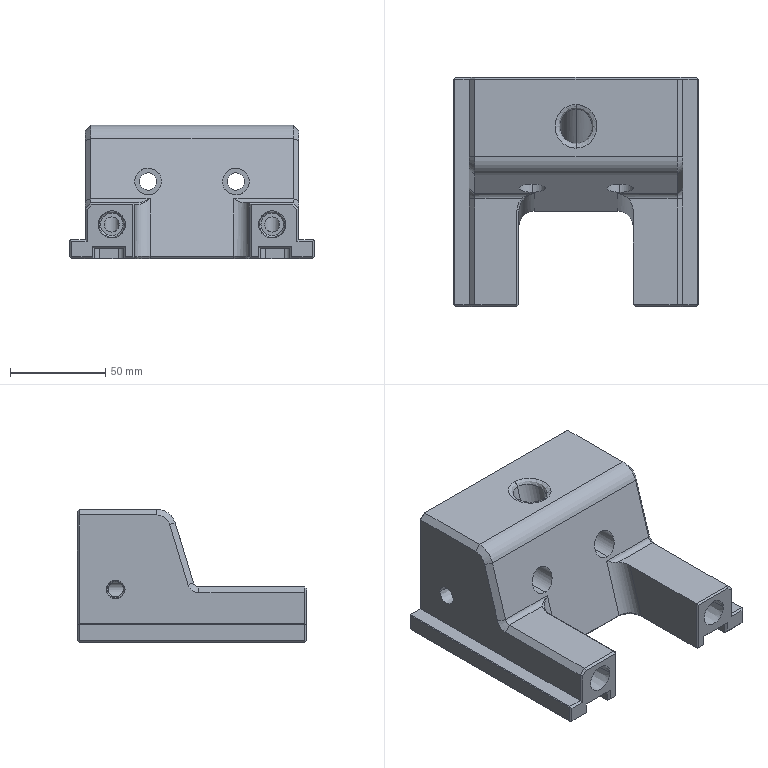Part | Creo | 1 solid | 197 faces | box 128 x 120 x 70 mm | volume 492365 mm3 | plane 98 | cylinder 61 | cone 28 | spline 6 | torus 4 | commonest cylinder face diameters 8 x26 6 x10 16 x6 1 x4 9 x4 9.4 x4